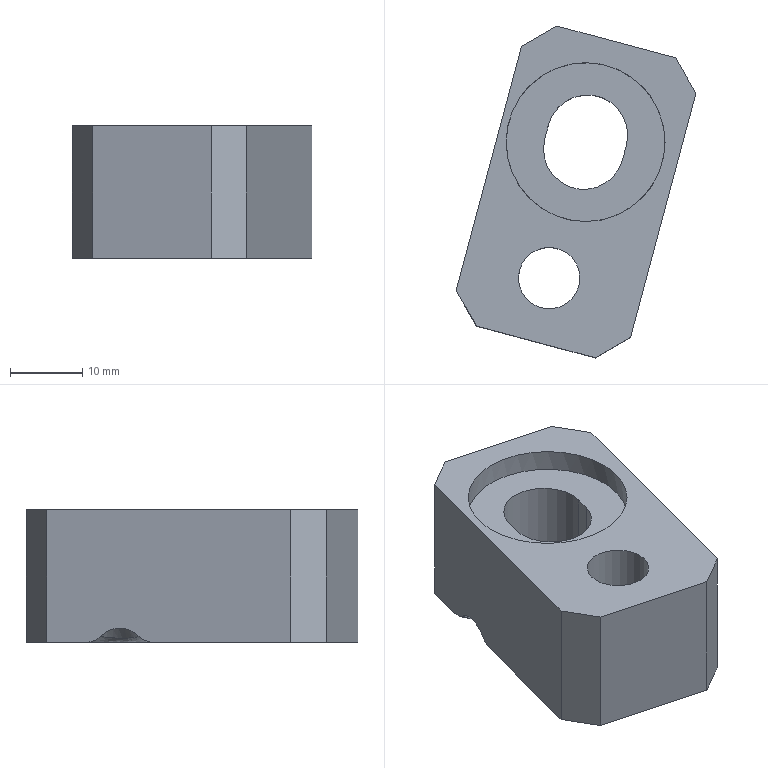Part | NX | features solid 2 | 1 solid | 21 faces | box 33.207 x 45.935 x 18.4 mm | volume 14179 mm3 | plane 14 | cylinder 6 | spline 1 | commonest cylinder face diameters 11.15 x2 8.5 x1 10 x1 14 x1 22 x1
STEP:
#1=CARTESIAN_POINT('',(1426.059,-51.189,5.));
#2=VERTEX_POINT('',#1);
#3=CARTESIAN_POINT('',(1421.809,-51.189,5.));
#4=DIRECTION('',(0.,0.,-1.));
#5=DIRECTION('',(1.,0.,0.));
#6=AXIS2_PLACEMENT_3D('',#3,#4,#5);
#7=CIRCLE('',#6,4.25);
#8=EDGE_CURVE('',#2,#2,#7,.T.);
#9=ORIENTED_EDGE('',*,*,#8,.T.);
#10=EDGE_LOOP('',(#9));
#11=FACE_BOUND('',#10,.T.);
#12=CARTESIAN_POINT('',(1408.924,-52.912,5.));
#13=VERTEX_POINT('',#12);
#14=CARTESIAN_POINT('',(1417.983,-19.105,5.));
#15=VERTEX_POINT('',#14);
#16=CARTESIAN_POINT('',(1407.889,-56.776,5.));
#17=DIRECTION('',(0.2588,0.9659,0.));
#18=VECTOR('',#17,1000.);
#19=LINE('',#16,#18);
#20=EDGE_CURVE('',#13,#15,#19,.T.);
#21=ORIENTED_EDGE('',*,*,#20,.F.);
#22=CARTESIAN_POINT('',(1411.752,-57.811,5.));
#23=VERTEX_POINT('',#22);
#24=CARTESIAN_POINT('',(1033.781,596.854,5.));
#25=DIRECTION('',(0.5,-0.866,0.));
#26=VECTOR('',#25,1000.);
#27=LINE('',#24,#26);
#28=EDGE_CURVE('',#23,#13,#27,.F.);
#29=ORIENTED_EDGE('',*,*,#28,.F.);
#30=CARTESIAN_POINT('',(1428.173,-62.211,5.));
#31=VERTEX_POINT('',#30);
#32=CARTESIAN_POINT('',(1432.037,-63.247,5.));
#33=DIRECTION('',(-0.9659,0.2588,0.));
#34=VECTOR('',#33,1000.);
#35=LINE('',#32,#34);
#36=EDGE_CURVE('',#31,#23,#35,.T.);
#37=ORIENTED_EDGE('',*,*,#36,.F.);
#38=CARTESIAN_POINT('',(1433.072,-59.383,5.));
#39=VERTEX_POINT('',#38);
#40=CARTESIAN_POINT('',(383.982,-665.076,5.));
#41=DIRECTION('',(0.866,0.5,0.));
#42=VECTOR('',#41,1000.);
#43=LINE('',#40,#42);
#44=EDGE_CURVE('',#39,#31,#43,.F.);
#45=ORIENTED_EDGE('',*,*,#44,.F.);
#46=CARTESIAN_POINT('',(1442.131,-25.575,5.));
#47=VERTEX_POINT('',#46);
#48=CARTESIAN_POINT('',(1443.425,-20.746,5.));
#49=DIRECTION('',(-0.2588,-0.9659,0.));
#50=VECTOR('',#49,1000.);
#51=LINE('',#48,#50);
#52=EDGE_CURVE('',#47,#39,#51,.T.);
#53=ORIENTED_EDGE('',*,*,#52,.F.);
#54=CARTESIAN_POINT('',(1439.302,-20.676,5.));
#55=VERTEX_POINT('',#54);
#56=CARTESIAN_POINT('',(1070.877,617.455,5.));
#57=DIRECTION('',(0.5,-0.866,0.));
#58=VECTOR('',#57,1000.);
#59=LINE('',#56,#58);
#60=EDGE_CURVE('',#55,#47,#59,.T.);
#61=ORIENTED_EDGE('',*,*,#60,.F.);
#62=CARTESIAN_POINT('',(1422.882,-16.277,5.));
#63=VERTEX_POINT('',#62);
#64=CARTESIAN_POINT('',(1419.018,-15.241,5.));
#65=DIRECTION('',(0.9659,-0.2588,0.));
#66=VECTOR('',#65,1000.);
#67=LINE('',#64,#66);
#68=EDGE_CURVE('',#63,#55,#67,.T.);
#69=ORIENTED_EDGE('',*,*,#68,.F.);
#70=CARTESIAN_POINT('',(362.156,-628.687,5.));
#71=DIRECTION('',(0.866,0.5,0.));
#72=VECTOR('',#71,1000.);
#73=LINE('',#70,#72);
#74=EDGE_CURVE('',#15,#63,#73,.T.);
#75=ORIENTED_EDGE('',*,*,#74,.F.);
#76=EDGE_LOOP('',(#21,#29,#37,#45,#53,#61,#69,#75));
#77=FACE_BOUND('',#76,.T.);
#78=CARTESIAN_POINT('',(1437.856,-32.353,5.));
#79=VERTEX_POINT('',#78);
#80=CARTESIAN_POINT('',(1426.856,-32.353,5.));
#81=DIRECTION('',(0.,0.,-1.));
#82=DIRECTION('',(1.,0.,0.));
#83=AXIS2_PLACEMENT_3D('',#80,#81,#82);
#84=CIRCLE('',#83,11.);
#85=EDGE_CURVE('',#79,#79,#84,.F.);
#86=ORIENTED_EDGE('',*,*,#85,.F.);
#87=EDGE_LOOP('',(#86));
#88=FACE_BOUND('',#87,.T.);
#89=CARTESIAN_POINT('',(0.,0.,5.));
#90=DIRECTION('',(0.,0.,1.));
#91=DIRECTION('',(1.,0.,0.));
#92=AXIS2_PLACEMENT_3D('',#89,#90,#91);
#93=PLANE('',#92);
#94=ADVANCED_FACE('',(#11,#77,#88),#93,.T.);
#95=ORIENTED_EDGE('',*,*,#85,.T.);
#96=EDGE_LOOP('',(#95));
#97=FACE_BOUND('',#96,.T.);
#98=CARTESIAN_POINT('',(1415.856,-32.353,2.));
#99=VERTEX_POINT('',#98);
#100=CARTESIAN_POINT('',(1426.856,-32.353,2.));
#101=DIRECTION('',(0.,0.,-1.));
#102=DIRECTION('',(-1.,0.,0.));
#103=AXIS2_PLACEMENT_3D('',#100,#101,#102);
#104=CIRCLE('',#103,11.);
#105=EDGE_CURVE('',#99,#99,#104,.T.);
#106=ORIENTED_EDGE('',*,*,#105,.T.);
#107=EDGE_LOOP('',(#106));
#108=FACE_BOUND('',#107,.T.);
#109=CARTESIAN_POINT('',(1426.856,-32.353,258.));
#110=DIRECTION('',(0.,0.,-1.));
#111=DIRECTION('',(-1.,0.,0.));
#112=AXIS2_PLACEMENT_3D('',#109,#110,#111);
#113=CYLINDRICAL_SURFACE('',#112,11.);
#114=ADVANCED_FACE('',(#97,#108),#113,.F.);
#115=CARTESIAN_POINT('',(1431.982,-34.762,2.));
#116=VERTEX_POINT('',#115);
#117=CARTESIAN_POINT('',(1431.982,-34.762,-13.4));
#118=VERTEX_POINT('',#117);
#119=CARTESIAN_POINT('',(1431.982,-34.762,-16.4));
#120=DIRECTION('',(0.,0.,1.));
#121=VECTOR('',#120,1000.);
#122=LINE('',#119,#121);
#123=EDGE_CURVE('',#116,#118,#122,.F.);
#124=ORIENTED_EDGE('',*,*,#123,.F.);
#125=CARTESIAN_POINT('',(1432.5,-32.83,2.));
#126=VERTEX_POINT('',#125);
#127=CARTESIAN_POINT('',(1429.265,-44.904,2.));
#128=DIRECTION('',(-0.2588,-0.9659,0.));
#129=VECTOR('',#128,1000.);
#130=LINE('',#127,#129);
#131=EDGE_CURVE('',#116,#126,#130,.F.);
#132=ORIENTED_EDGE('',*,*,#131,.T.);
#133=CARTESIAN_POINT('',(1432.5,-32.83,-13.4));
#134=VERTEX_POINT('',#133);
#135=CARTESIAN_POINT('',(1432.5,-32.83,-16.4));
#136=DIRECTION('',(0.,0.,1.));
#137=VECTOR('',#136,1000.);
#138=LINE('',#135,#137);
#139=EDGE_CURVE('',#126,#134,#138,.F.);
#140=ORIENTED_EDGE('',*,*,#139,.T.);
#141=CARTESIAN_POINT('',(1429.265,-44.904,-13.4));
#142=DIRECTION('',(-0.2588,-0.9659,0.));
#143=VECTOR('',#142,1000.);
#144=LINE('',#141,#143);
#145=EDGE_CURVE('',#118,#134,#144,.F.);
#146=ORIENTED_EDGE('',*,*,#145,.F.);
#147=EDGE_LOOP('',(#124,#132,#140,#146));
#148=FACE_BOUND('',#147,.T.);
#149=CARTESIAN_POINT('',(1429.265,-44.904,-16.4));
#150=DIRECTION('',(-0.9659,0.2588,0.));
#151=DIRECTION('',(0.2588,0.9659,0.));
#152=AXIS2_PLACEMENT_3D('',#149,#150,#151);
#153=PLANE('',#152);
#154=ADVANCED_FACE('',(#148),#153,.T.);
#155=ORIENTED_EDGE('',*,*,#139,.F.);
#156=CARTESIAN_POINT('',(1421.73,-29.944,2.));
#157=VERTEX_POINT('',#156);
#158=CARTESIAN_POINT('',(1427.115,-31.387,2.));
#159=DIRECTION('',(0.,0.,-1.));
#160=DIRECTION('',(-1.,0.,0.));
#161=AXIS2_PLACEMENT_3D('',#158,#159,#160);
#162=CIRCLE('',#161,5.575);
#163=EDGE_CURVE('',#157,#126,#162,.T.);
#164=ORIENTED_EDGE('',*,*,#163,.F.);
#165=CARTESIAN_POINT('',(1421.73,-29.944,-13.4));
#166=VERTEX_POINT('',#165);
#167=CARTESIAN_POINT('',(1421.73,-29.944,-16.4));
#168=DIRECTION('',(0.,0.,1.));
#169=VECTOR('',#168,1000.);
#170=LINE('',#167,#169);
#171=EDGE_CURVE('',#157,#166,#170,.F.);
#172=ORIENTED_EDGE('',*,*,#171,.T.);
#173=CARTESIAN_POINT('',(1427.115,-31.387,-13.4));
#174=DIRECTION('',(0.,0.,-1.));
#175=DIRECTION('',(1.,0.,0.));
#176=AXIS2_PLACEMENT_3D('',#173,#174,#175);
#177=CIRCLE('',#176,5.575);
#178=EDGE_CURVE('',#134,#166,#177,.F.);
#179=ORIENTED_EDGE('',*,*,#178,.F.);
#180=EDGE_LOOP('',(#155,#164,#172,#179));
#181=FACE_BOUND('',#180,.T.);
#182=CARTESIAN_POINT('',(1427.115,-31.387,-16.4));
#183=DIRECTION('',(0.,0.,1.));
#184=DIRECTION('',(1.,0.,0.));
#185=AXIS2_PLACEMENT_3D('',#182,#183,#184);
#186=CYLINDRICAL_SURFACE('',#185,5.575);
#187=ADVANCED_FACE('',(#181),#186,.F.);
#188=ORIENTED_EDGE('',*,*,#171,.F.);
#189=CARTESIAN_POINT('',(1421.212,-31.876,2.));
#190=VERTEX_POINT('',#189);
#191=CARTESIAN_POINT('',(1418.495,-42.018,2.));
#192=DIRECTION('',(0.2588,0.9659,0.));
#193=VECTOR('',#192,1000.);
#194=LINE('',#191,#193);
#195=EDGE_CURVE('',#157,#190,#194,.F.);
#196=ORIENTED_EDGE('',*,*,#195,.T.);
#197=CARTESIAN_POINT('',(1421.212,-31.876,-13.4));
#198=VERTEX_POINT('',#197);
#199=CARTESIAN_POINT('',(1421.212,-31.876,-16.4));
#200=DIRECTION('',(0.,0.,1.));
#201=VECTOR('',#200,1000.);
#202=LINE('',#199,#201);
#203=EDGE_CURVE('',#190,#198,#202,.F.);
#204=ORIENTED_EDGE('',*,*,#203,.T.);
#205=CARTESIAN_POINT('',(1418.495,-42.018,-13.4));
#206=DIRECTION('',(0.2588,0.9659,0.));
#207=VECTOR('',#206,1000.);
#208=LINE('',#205,#207);
#209=EDGE_CURVE('',#166,#198,#208,.F.);
#210=ORIENTED_EDGE('',*,*,#209,.F.);
#211=EDGE_LOOP('',(#188,#196,#204,#210));
#212=FACE_BOUND('',#211,.T.);
#213=CARTESIAN_POINT('',(1418.495,-42.018,-16.4));
#214=DIRECTION('',(0.9659,-0.2588,0.));
#215=DIRECTION('',(-0.2588,-0.9659,0.));
#216=AXIS2_PLACEMENT_3D('',#213,#214,#215);
#217=PLANE('',#216);
#218=ADVANCED_FACE('',(#212),#217,.T.);
#219=CARTESIAN_POINT('',(1433.072,-59.383,-13.4));
#220=VERTEX_POINT('',#219);
#221=CARTESIAN_POINT('',(1442.131,-25.575,-13.4));
#222=VERTEX_POINT('',#221);
#223=CARTESIAN_POINT('',(1436.437,-46.826,-13.4));
#224=DIRECTION('',(-0.2588,-0.9659,0.));
#225=VECTOR('',#224,1000.);
#226=LINE('',#223,#225);
#227=EDGE_CURVE('',#220,#222,#226,.F.);
#228=ORIENTED_EDGE('',*,*,#227,.T.);
#229=CARTESIAN_POINT('',(1442.131,-25.575,-16.4));
#230=DIRECTION('',(0.,0.,1.));
#231=VECTOR('',#230,1000.);
#232=LINE('',#229,#231);
#233=EDGE_CURVE('',#47,#222,#232,.F.);
#234=ORIENTED_EDGE('',*,*,#233,.F.);
#235=ORIENTED_EDGE('',*,*,#52,.T.);
#236=CARTESIAN_POINT('',(1433.072,-59.383,-16.4));
#237=DIRECTION('',(0.,0.,-1.));
#238=VECTOR('',#237,1000.);
#239=LINE('',#236,#238);
#240=EDGE_CURVE('',#220,#39,#239,.F.);
#241=ORIENTED_EDGE('',*,*,#240,.F.);
#242=EDGE_LOOP('',(#228,#234,#235,#241));
#243=FACE_BOUND('',#242,.T.);
#244=CARTESIAN_POINT('',(1436.437,-46.826,-16.4));
#245=DIRECTION('',(0.9659,-0.2588,0.));
#246=DIRECTION('',(-0.2588,-0.9659,0.));
#247=AXIS2_PLACEMENT_3D('',#244,#245,#246);
#248=PLANE('',#247);
#249=ADVANCED_FACE('',(#243),#248,.T.);
#250=CARTESIAN_POINT('',(1411.752,-57.811,-13.4));
#251=VERTEX_POINT('',#250);
#252=CARTESIAN_POINT('',(1428.173,-62.211,-13.4));
#253=VERTEX_POINT('',#252);
#254=CARTESIAN_POINT('',(1405.957,-56.258,-13.4));
#255=DIRECTION('',(-0.9659,0.2588,0.));
#256=VECTOR('',#255,1000.);
#257=LINE('',#254,#256);
#258=EDGE_CURVE('',#251,#253,#257,.F.);
#259=ORIENTED_EDGE('',*,*,#258,.T.);
#260=CARTESIAN_POINT('',(1428.173,-62.211,-16.4));
#261=DIRECTION('',(0.,0.,1.));
#262=VECTOR('',#261,1000.);
#263=LINE('',#260,#262);
#264=EDGE_CURVE('',#31,#253,#263,.F.);
#265=ORIENTED_EDGE('',*,*,#264,.F.);
#266=ORIENTED_EDGE('',*,*,#36,.T.);
#267=CARTESIAN_POINT('',(1411.752,-57.811,-16.4));
#268=DIRECTION('',(0.,0.,-1.));
#269=VECTOR('',#268,1000.);
#270=LINE('',#267,#269);
#271=EDGE_CURVE('',#251,#23,#270,.F.);
#272=ORIENTED_EDGE('',*,*,#271,.F.);
#273=EDGE_LOOP('',(#259,#265,#266,#272));
#274=FACE_BOUND('',#273,.T.);
#275=CARTESIAN_POINT('',(1405.957,-56.258,-16.4));
#276=DIRECTION('',(-0.2588,-0.9659,0.));
#277=DIRECTION('',(-0.9659,0.2588,0.));
#278=AXIS2_PLACEMENT_3D('',#275,#276,#277);
#279=PLANE('',#278);
#280=ADVANCED_FACE('',(#274),#279,.T.);
#281=CARTESIAN_POINT('',(1416.533,-24.515,-13.4));
#282=VERTEX_POINT('',#281);
#283=CARTESIAN_POINT('',(1417.983,-19.105,-13.4));
#284=VERTEX_POINT('',#283);
#285=CARTESIAN_POINT('',(1413.255,-36.748,-13.4));
#286=DIRECTION('',(-0.2588,-0.9659,0.));
#287=VECTOR('',#286,1000.);
#288=LINE('',#285,#287);
#289=EDGE_CURVE('',#282,#284,#288,.F.);
#290=ORIENTED_EDGE('',*,*,#289,.F.);
#291=CARTESIAN_POINT('',(1415.98,-26.578,-12.578));
#292=VERTEX_POINT('',#291);
#293=CARTESIAN_POINT('',(1415.98,-26.578,-12.579));
#294=CARTESIAN_POINT('',(1416.129,-26.023,-13.117));
#295=CARTESIAN_POINT('',(1416.33,-25.274,-13.4));
#296=CARTESIAN_POINT('',(1416.533,-24.515,-13.4));
#297=B_SPLINE_CURVE_WITH_KNOTS('',3,(#293,#294,#295,#296),.UNSPECIFIED.,.F.,.F.,(4,4),(0.,0.002325),.UNSPECIFIED.);
#298=EDGE_CURVE('',#292,#282,#297,.T.);
#299=ORIENTED_EDGE('',*,*,#298,.F.);
#300=CARTESIAN_POINT('',(1414.55,-31.917,-12.578));
#301=VERTEX_POINT('',#300);
#302=CARTESIAN_POINT('',(1415.265,-29.247,-18.471));
#303=DIRECTION('',(0.9659,-0.2588,0.));
#304=DIRECTION('',(0.,0.,1.));
#305=AXIS2_PLACEMENT_3D('',#302,#303,#304);
#306=ELLIPSE('',#305,7.071,5.);
#307=EDGE_CURVE('',#301,#292,#306,.F.);
#308=ORIENTED_EDGE('',*,*,#307,.F.);
#309=CARTESIAN_POINT('',(1413.997,-33.979,-13.4));
#310=VERTEX_POINT('',#309);
#311=CARTESIAN_POINT('',(1413.997,-33.979,-13.4));
#312=CARTESIAN_POINT('',(1414.201,-33.219,-13.4));
#313=CARTESIAN_POINT('',(1414.401,-32.472,-13.117));
#314=CARTESIAN_POINT('',(1414.55,-31.917,-12.579));
#315=B_SPLINE_CURVE_WITH_KNOTS('',3,(#311,#312,#313,#314),.UNSPECIFIED.,.F.,.F.,(4,4),(0.,0.002329),.UNSPECIFIED.);
#316=EDGE_CURVE('',#310,#301,#315,.T.);
#317=ORIENTED_EDGE('',*,*,#316,.F.);
#318=CARTESIAN_POINT('',(1408.924,-52.912,-13.4));
#319=VERTEX_POINT('',#318);
#320=CARTESIAN_POINT('',(1413.255,-36.748,-13.4));
#321=DIRECTION('',(-0.2588,-0.9659,0.));
#322=VECTOR('',#321,1000.);
#323=LINE('',#320,#322);
#324=EDGE_CURVE('',#319,#310,#323,.F.);
#325=ORIENTED_EDGE('',*,*,#324,.F.);
#326=CARTESIAN_POINT('',(1408.924,-52.912,-16.4));
#327=DIRECTION('',(0.,0.,1.));
#328=VECTOR('',#327,1000.);
#329=LINE('',#326,#328);
#330=EDGE_CURVE('',#13,#319,#329,.F.);
#331=ORIENTED_EDGE('',*,*,#330,.F.);
#332=ORIENTED_EDGE('',*,*,#20,.T.);
#333=CARTESIAN_POINT('',(1417.983,-19.105,-16.4));
#334=DIRECTION('',(0.,0.,-1.));
#335=VECTOR('',#334,1000.);
#336=LINE('',#333,#335);
#337=EDGE_CURVE('',#284,#15,#336,.F.);
#338=ORIENTED_EDGE('',*,*,#337,.F.);
#339=EDGE_LOOP('',(#290,#299,#308,#317,#325,#331,#332,#338));
#340=FACE_BOUND('',#339,.T.);
#341=CARTESIAN_POINT('',(1413.255,-36.748,-16.4));
#342=DIRECTION('',(-0.9659,0.2588,0.));
#343=DIRECTION('',(0.2588,0.9659,0.));
#344=AXIS2_PLACEMENT_3D('',#341,#342,#343);
#345=PLANE('',#344);
#346=ADVANCED_FACE('',(#340),#345,.T.);
#347=ORIENTED_EDGE('',*,*,#68,.T.);
#348=CARTESIAN_POINT('',(1439.302,-20.676,-13.4));
#349=VERTEX_POINT('',#348);
#350=CARTESIAN_POINT('',(1439.302,-20.676,-16.4));
#351=DIRECTION('',(0.,0.,1.));
#352=VECTOR('',#351,1000.);
#353=LINE('',#350,#352);
#354=EDGE_CURVE('',#349,#55,#353,.T.);
#355=ORIENTED_EDGE('',*,*,#354,.F.);
#356=CARTESIAN_POINT('',(1422.882,-16.277,-13.4));
#357=VERTEX_POINT('',#356);
#358=CARTESIAN_POINT('',(1417.086,-14.724,-13.4));
#359=DIRECTION('',(0.9659,-0.2588,0.));
#360=VECTOR('',#359,1000.);
#361=LINE('',#358,#360);
#362=EDGE_CURVE('',#357,#349,#361,.T.);
#363=ORIENTED_EDGE('',*,*,#362,.F.);
#364=CARTESIAN_POINT('',(1422.882,-16.277,-16.4));
#365=DIRECTION('',(0.,0.,-1.));
#366=VECTOR('',#365,1000.);
#367=LINE('',#364,#366);
#368=EDGE_CURVE('',#63,#357,#367,.T.);
#369=ORIENTED_EDGE('',*,*,#368,.F.);
#370=EDGE_LOOP('',(#347,#355,#363,#369));
#371=FACE_BOUND('',#370,.T.);
#372=CARTESIAN_POINT('',(1417.086,-14.724,-16.4));
#373=DIRECTION('',(-0.2588,-0.9659,0.));
#374=DIRECTION('',(-0.9659,0.2588,0.));
#375=AXIS2_PLACEMENT_3D('',#372,#373,#374);
#376=PLANE('',#375);
#377=ADVANCED_FACE('',(#371),#376,.F.);
#378=ORIENTED_EDGE('',*,*,#203,.F.);
#379=CARTESIAN_POINT('',(1426.597,-33.319,2.));
#380=DIRECTION('',(0.,0.,-1.));
#381=DIRECTION('',(-1.,0.,0.));
#382=AXIS2_PLACEMENT_3D('',#379,#380,#381);
#383=CIRCLE('',#382,5.575);
#384=EDGE_CURVE('',#116,#190,#383,.T.);
#385=ORIENTED_EDGE('',*,*,#384,.F.);
#386=ORIENTED_EDGE('',*,*,#123,.T.);
#387=CARTESIAN_POINT('',(1426.597,-33.319,-13.4));
#388=DIRECTION('',(0.,0.,-1.));
#389=DIRECTION('',(1.,0.,0.));
#390=AXIS2_PLACEMENT_3D('',#387,#388,#389);
#391=CIRCLE('',#390,5.575);
#392=EDGE_CURVE('',#198,#118,#391,.F.);
#393=ORIENTED_EDGE('',*,*,#392,.F.);
#394=EDGE_LOOP('',(#378,#385,#386,#393));
#395=FACE_BOUND('',#394,.T.);
#396=CARTESIAN_POINT('',(1426.597,-33.319,-16.4));
#397=DIRECTION('',(0.,0.,1.));
#398=DIRECTION('',(1.,0.,0.));
#399=AXIS2_PLACEMENT_3D('',#396,#397,#398);
#400=CYLINDRICAL_SURFACE('',#399,5.575);
#401=ADVANCED_FACE('',(#395),#400,.F.);
#402=CARTESIAN_POINT('',(1428.809,-51.189,-13.4));
#403=VERTEX_POINT('',#402);
#404=CARTESIAN_POINT('',(1421.809,-51.189,-13.4));
#405=DIRECTION('',(0.,0.,-1.));
#406=DIRECTION('',(1.,0.,0.));
#407=AXIS2_PLACEMENT_3D('',#404,#405,#406);
#408=CIRCLE('',#407,7.);
#409=EDGE_CURVE('',#403,#403,#408,.T.);
#410=ORIENTED_EDGE('',*,*,#409,.F.);
#411=EDGE_LOOP('',(#410));
#412=FACE_BOUND('',#411,.T.);
#413=ORIENTED_EDGE('',*,*,#362,.T.);
#414=CARTESIAN_POINT('',(1439.302,-20.676,-13.4));
#415=DIRECTION('',(-0.5,0.866,0.));
#416=VECTOR('',#415,1000.);
#417=LINE('',#414,#416);
#418=EDGE_CURVE('',#222,#349,#417,.T.);
#419=ORIENTED_EDGE('',*,*,#418,.F.);
#420=ORIENTED_EDGE('',*,*,#227,.F.);
#421=CARTESIAN_POINT('',(1433.072,-59.383,-13.4));
#422=DIRECTION('',(-0.866,-0.5,0.));
#423=VECTOR('',#422,1000.);
#424=LINE('',#421,#423);
#425=EDGE_CURVE('',#253,#220,#424,.F.);
#426=ORIENTED_EDGE('',*,*,#425,.F.);
#427=ORIENTED_EDGE('',*,*,#258,.F.);
#428=CARTESIAN_POINT('',(1411.752,-57.811,-13.4));
#429=DIRECTION('',(-0.5,0.866,0.));
#430=VECTOR('',#429,1000.);
#431=LINE('',#428,#430);
#432=EDGE_CURVE('',#319,#251,#431,.F.);
#433=ORIENTED_EDGE('',*,*,#432,.F.);
#434=ORIENTED_EDGE('',*,*,#324,.T.);
#435=CARTESIAN_POINT('',(1413.997,-33.979,-13.4));
#436=CARTESIAN_POINT('',(1414.228,-33.891,-13.4));
#437=CARTESIAN_POINT('',(1414.564,-33.748,-13.4));
#438=CARTESIAN_POINT('',(1414.934,-33.559,-13.4));
#439=CARTESIAN_POINT('',(1415.115,-33.46,-13.4));
#440=CARTESIAN_POINT('',(1415.204,-33.409,-13.4));
#441=CARTESIAN_POINT('',(1415.241,-33.387,-13.4));
#442=CARTESIAN_POINT('',(1415.266,-33.372,-13.4));
#443=CARTESIAN_POINT('',(1415.278,-33.365,-13.4));
#444=CARTESIAN_POINT('',(1415.508,-33.228,-13.4));
#445=CARTESIAN_POINT('',(1415.815,-33.022,-13.4));
#446=CARTESIAN_POINT('',(1416.146,-32.761,-13.4));
#447=CARTESIAN_POINT('',(1416.304,-32.625,-13.4));
#448=CARTESIAN_POINT('',(1416.381,-32.556,-13.4));
#449=CARTESIAN_POINT('',(1416.414,-32.526,-13.4));
#450=CARTESIAN_POINT('',(1416.436,-32.506,-13.4));
#451=CARTESIAN_POINT('',(1416.446,-32.497,-13.4));
#452=CARTESIAN_POINT('',(1416.643,-32.312,-13.4));
#453=CARTESIAN_POINT('',(1416.901,-32.039,-13.4));
#454=CARTESIAN_POINT('',(1417.163,-31.7,-13.4));
#455=CARTESIAN_POINT('',(1417.284,-31.526,-13.4));
#456=CARTESIAN_POINT('',(1417.335,-31.45,-13.4));
#457=CARTESIAN_POINT('',(1417.367,-31.399,-13.4));
#458=CARTESIAN_POINT('',(1417.383,-31.375,-13.4));
#459=CARTESIAN_POINT('',(1417.669,-30.917,-13.4));
#460=CARTESIAN_POINT('',(1417.868,-30.46,-13.4));
#461=CARTESIAN_POINT('',(1418.061,-29.739,-13.4));
#462=CARTESIAN_POINT('',(1418.131,-29.374,-13.4));
#463=CARTESIAN_POINT('',(1418.163,-28.938,-13.4));
#464=CARTESIAN_POINT('',(1418.168,-28.717,-13.4));
#465=CARTESIAN_POINT('',(1418.167,-28.623,-13.4));
#466=CARTESIAN_POINT('',(1418.166,-28.559,-13.4));
#467=CARTESIAN_POINT('',(1418.165,-28.526,-13.4));
#468=CARTESIAN_POINT('',(1418.156,-28.254,-13.4));
#469=CARTESIAN_POINT('',(1418.119,-27.891,-13.4));
#470=CARTESIAN_POINT('',(1418.032,-27.466,-13.4));
#471=CARTESIAN_POINT('',(1417.978,-27.252,-13.4));
#472=CARTESIAN_POINT('',(1417.948,-27.146,-13.4));
#473=CARTESIAN_POINT('',(1417.935,-27.1,-13.4));
#474=CARTESIAN_POINT('',(1417.926,-27.069,-13.4));
#475=CARTESIAN_POINT('',(1417.921,-27.053,-13.4));
#476=CARTESIAN_POINT('',(1417.848,-26.813,-13.4));
#477=CARTESIAN_POINT('',(1417.725,-26.476,-13.4));
#478=CARTESIAN_POINT('',(1417.546,-26.087,-13.4));
#479=CARTESIAN_POINT('',(1417.447,-25.894,-13.4));
#480=CARTESIAN_POINT('',(1417.396,-25.797,-13.4));
#481=CARTESIAN_POINT('',(1417.373,-25.756,-13.4));
#482=CARTESIAN_POINT('',(1417.358,-25.728,-13.4));
#483=CARTESIAN_POINT('',(1417.35,-25.713,-13.4));
#484=CARTESIAN_POINT('',(1417.116,-25.294,-13.4));
#485=CARTESIAN_POINT('',(1416.846,-24.899,-13.4));
#486=CARTESIAN_POINT('',(1416.533,-24.515,-13.4));
#487=B_SPLINE_CURVE_WITH_KNOTS('',3,(#435,#436,#437,#438,#439,#440,#441,#442,#443,#444,#445,#446,#447,#448,#449,#450,#451,#452,#453,#454,#455,#456,#457,#458,#459,#460,#461,#462,#463,#464,#465,#466,#467,#468,#469,#470,#471,#472,#473,#474,#475,#476,#477,#478,#479,#480,#481,#482,#483,#484,#485,#486),.UNSPECIFIED.,.F.,.F.,(4,1,1,1,1,2,2,1,1,1,1,2,2,1,1,1,2,2,2,1,1,1,2,2,1,1,1,1,2,2,1,1,1,1,2,2,4),(0.,0.0625,0.09375,0.1094,0.1172,0.1211,0.125,0.1875,0.2187,0.2344,0.2422,0.2461,0.25,0.3125,0.3437,0.3594,0.3672,0.375,0.5,0.5625,0.5937,0.6094,0.6172,0.625,0.6875,0.7187,0.7344,0.7422,0.7461,0.75,0.8125,0.8437,0.8594,0.8672,0.8711,0.875,1.),.UNSPECIFIED.);
#488=EDGE_CURVE('',#310,#282,#487,.T.);
#489=ORIENTED_EDGE('',*,*,#488,.T.);
#490=ORIENTED_EDGE('',*,*,#289,.T.);
#491=CARTESIAN_POINT('',(1417.983,-19.105,-13.4));
#492=DIRECTION('',(-0.866,-0.5,0.));
#493=VECTOR('',#492,1000.);
#494=LINE('',#491,#493);
#495=EDGE_CURVE('',#357,#284,#494,.T.);
#496=ORIENTED_EDGE('',*,*,#495,.F.);
#497=EDGE_LOOP('',(#413,#419,#420,#426,#427,#433,#434,#489,#490,#496));
#498=FACE_BOUND('',#497,.T.);
#499=ORIENTED_EDGE('',*,*,#209,.T.);
#500=ORIENTED_EDGE('',*,*,#392,.T.);
#501=ORIENTED_EDGE('',*,*,#145,.T.);
#502=ORIENTED_EDGE('',*,*,#178,.T.);
#503=EDGE_LOOP('',(#499,#500,#501,#502));
#504=FACE_BOUND('',#503,.T.);
#505=CARTESIAN_POINT('',(1410.357,-39.838,-13.4));
#506=DIRECTION('',(0.,0.,1.));
#507=DIRECTION('',(-0.2588,-0.9659,0.));
#508=AXIS2_PLACEMENT_3D('',#505,#506,#507);
#509=PLANE('',#508);
#510=ADVANCED_FACE('',(#412,#498,#504),#509,.F.);
#511=CARTESIAN_POINT('',(1416.631,-29.613,-12.814));
#512=VERTEX_POINT('',#511);
#513=CARTESIAN_POINT('',(1416.631,-29.613,-12.814));
#514=CARTESIAN_POINT('',(1416.5,-30.101,-12.814));
#515=CARTESIAN_POINT('',(1416.105,-30.8,-12.78));
#516=CARTESIAN_POINT('',(1415.232,-31.538,-12.672));
#517=CARTESIAN_POINT('',(1414.8,-31.791,-12.613));
#518=CARTESIAN_POINT('',(1414.55,-31.917,-12.578));
#519=B_SPLINE_CURVE_WITH_KNOTS('',3,(#513,#514,#515,#516,#517,#518),.UNSPECIFIED.,.F.,.F.,(4,1,1,4),(0.,0.3712,0.5568,0.7424),.UNSPECIFIED.);
#520=EDGE_CURVE('',#301,#512,#519,.F.);
#521=ORIENTED_EDGE('',*,*,#520,.F.);
#522=ORIENTED_EDGE('',*,*,#307,.T.);
#523=CARTESIAN_POINT('',(1415.98,-26.578,-12.578));
#524=CARTESIAN_POINT('',(1416.134,-26.811,-12.613));
#525=CARTESIAN_POINT('',(1416.382,-27.247,-12.672));
#526=CARTESIAN_POINT('',(1416.769,-28.322,-12.78));
#527=CARTESIAN_POINT('',(1416.762,-29.125,-12.814));
#528=CARTESIAN_POINT('',(1416.631,-29.613,-12.814));
#529=B_SPLINE_CURVE_WITH_KNOTS('',3,(#523,#524,#525,#526,#527,#528),.UNSPECIFIED.,.F.,.F.,(4,1,1,4),(0.2576,0.4432,0.6288,1.),.UNSPECIFIED.);
#530=EDGE_CURVE('',#512,#292,#529,.F.);
#531=ORIENTED_EDGE('',*,*,#530,.F.);
#532=EDGE_LOOP('',(#521,#522,#531));
#533=FACE_BOUND('',#532,.T.);
#534=CARTESIAN_POINT('',(1411.815,-28.323,-14.899));
#535=DIRECTION('',(-0.683,0.183,0.7071));
#536=DIRECTION('',(-0.683,0.183,-0.7071));
#537=AXIS2_PLACEMENT_3D('',#534,#535,#536);
#538=CYLINDRICAL_SURFACE('',#537,5.);
#539=ADVANCED_FACE('',(#533),#538,.F.);
#540=ORIENTED_EDGE('',*,*,#530,.T.);
#541=ORIENTED_EDGE('',*,*,#298,.T.);
#542=ORIENTED_EDGE('',*,*,#488,.F.);
#543=ORIENTED_EDGE('',*,*,#316,.T.);
#544=ORIENTED_EDGE('',*,*,#520,.T.);
#545=EDGE_LOOP('',(#540,#541,#542,#543,#544));
#546=FACE_BOUND('',#545,.T.);
#547=CARTESIAN_POINT('',(1413.384,-32.366,-12.41));
#548=CARTESIAN_POINT('',(1413.509,-32.696,-13.013));
#549=CARTESIAN_POINT('',(1413.753,-33.338,-13.4));
#550=CARTESIAN_POINT('',(1414.002,-33.991,-13.4));
#551=CARTESIAN_POINT('',(1414.126,-32.152,-12.521));
#552=CARTESIAN_POINT('',(1414.293,-32.485,-13.064));
#553=CARTESIAN_POINT('',(1414.591,-33.065,-13.4));
#554=CARTESIAN_POINT('',(1414.893,-33.651,-13.4));
#555=CARTESIAN_POINT('',(1414.833,-31.832,-12.62));
#556=CARTESIAN_POINT('',(1415.047,-32.147,-13.107));
#557=CARTESIAN_POINT('',(1415.396,-32.654,-13.4));
#558=CARTESIAN_POINT('',(1415.748,-33.165,-13.4));
#559=CARTESIAN_POINT('',(1415.998,-30.913,-12.768));
#560=CARTESIAN_POINT('',(1416.299,-31.148,-13.169));
#561=CARTESIAN_POINT('',(1416.739,-31.484,-13.4));
#562=CARTESIAN_POINT('',(1417.181,-31.822,-13.4));
#563=CARTESIAN_POINT('',(1416.446,-30.305,-12.814));
#564=CARTESIAN_POINT('',(1416.786,-30.474,-13.187));
#565=CARTESIAN_POINT('',(1417.265,-30.712,-13.4));
#566=CARTESIAN_POINT('',(1417.747,-30.952,-13.4));
#567=CARTESIAN_POINT('',(1416.816,-28.922,-12.814));
#568=CARTESIAN_POINT('',(1417.196,-28.946,-13.187));
#569=CARTESIAN_POINT('',(1417.73,-28.979,-13.4));
#570=CARTESIAN_POINT('',(1418.266,-29.013,-13.4));
#571=CARTESIAN_POINT('',(1416.733,-28.171,-12.768));
#572=CARTESIAN_POINT('',(1417.111,-28.119,-13.169));
#573=CARTESIAN_POINT('',(1417.66,-28.047,-13.4));
#574=CARTESIAN_POINT('',(1418.212,-27.976,-13.4));
#575=CARTESIAN_POINT('',(1416.183,-26.793,-12.62));
#576=CARTESIAN_POINT('',(1416.526,-26.627,-13.107));
#577=CARTESIAN_POINT('',(1417.082,-26.362,-13.4));
#578=CARTESIAN_POINT('',(1417.642,-26.096,-13.4));
#579=CARTESIAN_POINT('',(1415.732,-26.162,-12.521));
#580=CARTESIAN_POINT('',(1416.042,-25.957,-13.064));
#581=CARTESIAN_POINT('',(1416.59,-25.604,-13.4));
#582=CARTESIAN_POINT('',(1417.145,-25.247,-13.4));
#583=CARTESIAN_POINT('',(1415.195,-25.606,-12.41));
#584=CARTESIAN_POINT('',(1415.468,-25.383,-13.013));
#585=CARTESIAN_POINT('',(1416.002,-24.948,-13.4));
#586=CARTESIAN_POINT('',(1416.543,-24.507,-13.4));
#587=B_SPLINE_SURFACE_WITH_KNOTS('',3,3,((#547,#548,#549,#550),(#551,#552,#553,#554),(#555,#556,#557,#558),(#559,#560,#561,#562),(#563,#564,#565,#566),(#567,#568,#569,#570),(#571,#572,#573,#574),(#575,#576,#577,#578),(#579,#580,#581,#582),(#583,#584,#585,#586)),.UNSPECIFIED.,.F.,.F.,.F.,(4,2,2,2,4),(4,4),(0.,0.25,0.5,0.75,1.),(0.,1.006),.UNSPECIFIED.);
#588=ADVANCED_FACE('',(#546),#587,.T.);
#589=ORIENTED_EDGE('',*,*,#105,.F.);
#590=EDGE_LOOP('',(#589));
#591=FACE_BOUND('',#590,.T.);
#592=ORIENTED_EDGE('',*,*,#384,.T.);
#593=ORIENTED_EDGE('',*,*,#195,.F.);
#594=ORIENTED_EDGE('',*,*,#163,.T.);
#595=ORIENTED_EDGE('',*,*,#131,.F.);
#596=EDGE_LOOP('',(#592,#593,#594,#595));
#597=FACE_BOUND('',#596,.T.);
#598=CARTESIAN_POINT('',(1385.653,-55.777,2.));
#599=DIRECTION('',(0.,0.,-1.));
#600=DIRECTION('',(-1.,0.,0.));
#601=AXIS2_PLACEMENT_3D('',#598,#599,#600);
#602=PLANE('',#601);
#603=ADVANCED_FACE('',(#591,#597),#602,.F.);
#604=ORIENTED_EDGE('',*,*,#8,.F.);
#605=EDGE_LOOP('',(#604));
#606=FACE_BOUND('',#605,.T.);
#607=CARTESIAN_POINT('',(1426.059,-51.189,-3.4));
#608=VERTEX_POINT('',#607);
#609=CARTESIAN_POINT('',(1421.809,-51.189,-3.4));
#610=DIRECTION('',(0.,0.,-1.));
#611=DIRECTION('',(1.,0.,0.));
#612=AXIS2_PLACEMENT_3D('',#609,#610,#611);
#613=CIRCLE('',#612,4.25);
#614=EDGE_CURVE('',#608,#608,#613,.F.);
#615=ORIENTED_EDGE('',*,*,#614,.F.);
#616=EDGE_LOOP('',(#615));
#617=FACE_BOUND('',#616,.T.);
#618=CARTESIAN_POINT('',(1421.809,-51.189,336.6));
#619=DIRECTION('',(0.,0.,1.));
#620=DIRECTION('',(1.,0.,0.));
#621=AXIS2_PLACEMENT_3D('',#618,#619,#620);
#622=CYLINDRICAL_SURFACE('',#621,4.25);
#623=ADVANCED_FACE('',(#606,#617),#622,.F.);
#624=ORIENTED_EDGE('',*,*,#614,.T.);
#625=EDGE_LOOP('',(#624));
#626=FACE_BOUND('',#625,.T.);
#627=CARTESIAN_POINT('',(1428.809,-51.189,-3.4));
#628=VERTEX_POINT('',#627);
#629=CARTESIAN_POINT('',(1421.809,-51.189,-3.4));
#630=DIRECTION('',(0.,0.,-1.));
#631=DIRECTION('',(1.,0.,0.));
#632=AXIS2_PLACEMENT_3D('',#629,#630,#631);
#633=CIRCLE('',#632,7.);
#634=EDGE_CURVE('',#628,#628,#633,.F.);
#635=ORIENTED_EDGE('',*,*,#634,.F.);
#636=EDGE_LOOP('',(#635));
#637=FACE_BOUND('',#636,.T.);
#638=CARTESIAN_POINT('',(1420.85,-52.952,-3.4));
#639=DIRECTION('',(0.,0.,1.));
#640=DIRECTION('',(1.,0.,0.));
#641=AXIS2_PLACEMENT_3D('',#638,#639,#640);
#642=PLANE('',#641);
#643=ADVANCED_FACE('',(#626,#637),#642,.F.);
#644=ORIENTED_EDGE('',*,*,#634,.T.);
#645=EDGE_LOOP('',(#644));
#646=FACE_BOUND('',#645,.T.);
#647=ORIENTED_EDGE('',*,*,#409,.T.);
#648=EDGE_LOOP('',(#647));
#649=FACE_BOUND('',#648,.T.);
#650=CARTESIAN_POINT('',(1421.809,-51.189,-13.4));
#651=DIRECTION('',(0.,0.,1.));
#652=DIRECTION('',(1.,0.,0.));
#653=AXIS2_PLACEMENT_3D('',#650,#651,#652);
#654=CYLINDRICAL_SURFACE('',#653,7.);
#655=ADVANCED_FACE('',(#646,#649),#654,.F.);
#656=ORIENTED_EDGE('',*,*,#495,.T.);
#657=ORIENTED_EDGE('',*,*,#337,.T.);
#658=ORIENTED_EDGE('',*,*,#74,.T.);
#659=ORIENTED_EDGE('',*,*,#368,.T.);
#660=EDGE_LOOP('',(#656,#657,#658,#659));
#661=FACE_BOUND('',#660,.T.);
#662=CARTESIAN_POINT('',(1417.983,-19.105,-16.4));
#663=DIRECTION('',(-0.5,0.866,0.));
#664=DIRECTION('',(0.,0.,-1.));
#665=AXIS2_PLACEMENT_3D('',#662,#663,#664);
#666=PLANE('',#665);
#667=ADVANCED_FACE('',(#661),#666,.T.);
#668=ORIENTED_EDGE('',*,*,#432,.T.);
#669=ORIENTED_EDGE('',*,*,#271,.T.);
#670=ORIENTED_EDGE('',*,*,#28,.T.);
#671=ORIENTED_EDGE('',*,*,#330,.T.);
#672=EDGE_LOOP('',(#668,#669,#670,#671));
#673=FACE_BOUND('',#672,.T.);
#674=CARTESIAN_POINT('',(1411.752,-57.811,-16.4));
#675=DIRECTION('',(0.866,0.5,0.));
#676=DIRECTION('',(0.,0.,1.));
#677=AXIS2_PLACEMENT_3D('',#674,#675,#676);
#678=PLANE('',#677);
#679=ADVANCED_FACE('',(#673),#678,.F.);
#680=ORIENTED_EDGE('',*,*,#425,.T.);
#681=ORIENTED_EDGE('',*,*,#240,.T.);
#682=ORIENTED_EDGE('',*,*,#44,.T.);
#683=ORIENTED_EDGE('',*,*,#264,.T.);
#684=EDGE_LOOP('',(#680,#681,#682,#683));
#685=FACE_BOUND('',#684,.T.);
#686=CARTESIAN_POINT('',(1433.072,-59.383,-16.4));
#687=DIRECTION('',(-0.5,0.866,0.));
#688=DIRECTION('',(0.,0.,1.));
#689=AXIS2_PLACEMENT_3D('',#686,#687,#688);
#690=PLANE('',#689);
#691=ADVANCED_FACE('',(#685),#690,.F.);
#692=ORIENTED_EDGE('',*,*,#418,.T.);
#693=ORIENTED_EDGE('',*,*,#354,.T.);
#694=ORIENTED_EDGE('',*,*,#60,.T.);
#695=ORIENTED_EDGE('',*,*,#233,.T.);
#696=EDGE_LOOP('',(#692,#693,#694,#695));
#697=FACE_BOUND('',#696,.T.);
#698=CARTESIAN_POINT('',(1439.302,-20.676,-16.4));
#699=DIRECTION('',(0.866,0.5,0.));
#700=DIRECTION('',(0.,0.,-1.));
#701=AXIS2_PLACEMENT_3D('',#698,#699,#700);
#702=PLANE('',#701);
#703=ADVANCED_FACE('',(#697),#702,.T.);
#704=CLOSED_SHELL('',(#94,#114,#154,#187,#218,#249,#280,#346,#377,#401,#510,#539,#588,#603,#623,#643,#655,#667,#679,#691,#703));
#705=MANIFOLD_SOLID_BREP('',#704);
#706=(LENGTH_UNIT()NAMED_UNIT(*)SI_UNIT(.MILLI.,.METRE.));
#707=UNCERTAINTY_MEASURE_WITH_UNIT(LENGTH_MEASURE(0.0508),#706,'','');
#708=(NAMED_UNIT(*)PLANE_ANGLE_UNIT()SI_UNIT($,.RADIAN.));
#709=(NAMED_UNIT(*)SI_UNIT($,.STERADIAN.)SOLID_ANGLE_UNIT());
#710=(GEOMETRIC_REPRESENTATION_CONTEXT(3)GLOBAL_UNCERTAINTY_ASSIGNED_CONTEXT((#707))GLOBAL_UNIT_ASSIGNED_CONTEXT((#706,#708,#709))REPRESENTATION_CONTEXT('',''));
#711=ADVANCED_BREP_SHAPE_REPRESENTATION('',(#705),#710);